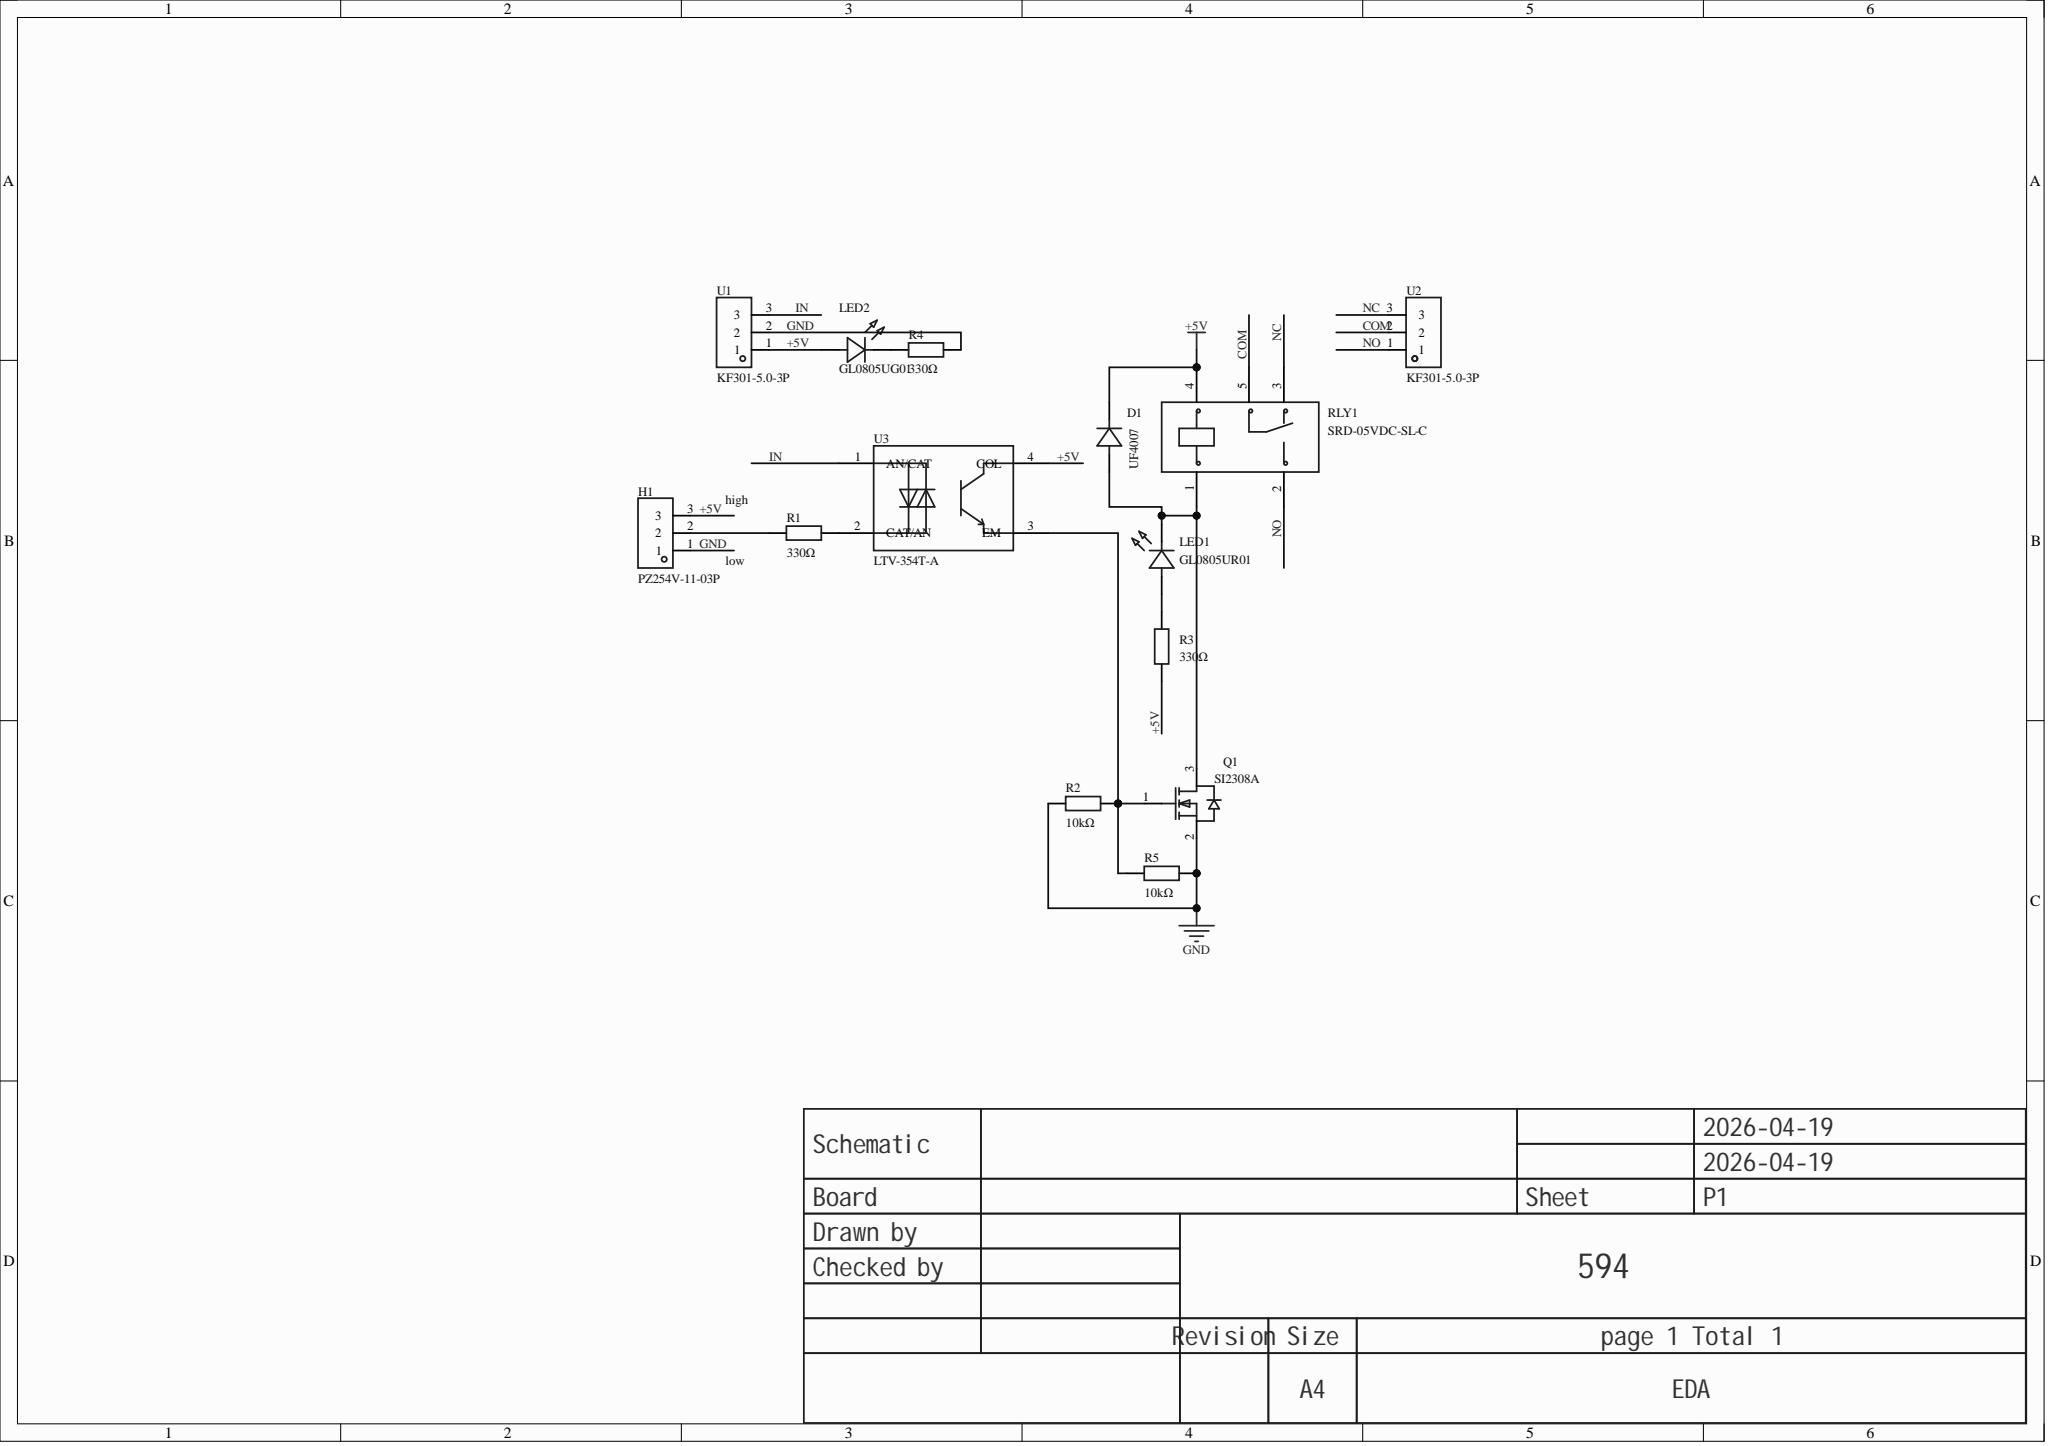Circuit board | Altium Designer | 14 parts | 12 nets
Bill of materials:
Comment,Description,Designator,Footprint,LibRef,Quantity
"UF4007","Diode configuration: -; forward voltage (Vf): 1.7V@1A; reverse breakdown voltage (Vr): 1kV; rectified current: 1A; reverse recovery time (Trr): 75ns;","D1","DO-41_BD2.4-L4.7-P8.70-D0.9-RD","UF4007_C960666","1"
"PZ254V-11-03P","","H1","HDR-TH_3P-P2.54-V-M_PZ254V-11-03P","PZ254V-11-03P","1"
"GL0805UR01","","LED1","LED0805-R-RD_RED","GL0805UR01","1"
"GL0805UG01","","LED2","LED0805-FD_GL0805UG01","GL0805UG01","1"
"SI2308A","Quantity: 1 N-channel; drain-source voltage (Vdss): 60V; continuous drain current (Id): 3A; on-resistance (RDS(on)): 80mΩ@10V; 95mΩ@4.5V; power dissipation (Pd): 1.25W; threshold voltage (Vgs(th)): 3V@250uA;","Q1","SOT-23-3_L2.9-W1.3-P1.90-LS2.4-BR","SI2308A","1"
"330Ω","Resistor type: thick film resistor; resistance: 330Ω; tolerance: ±1%; power: 100mW; max working voltage: 75V; temperature coefficient: ±100ppm/?;","R1, R3, R4","R0603","0603WAF3300T5E","3"
"10kΩ","Resistor type: thick film resistor; resistance: 10kΩ; tolerance: ±5%; power: 100mW; max working voltage: 75V; temperature coefficient: ±100ppm/?;","R2, R5","R0603","0603WAJ0103T5E","2"
"SRD-05VDC-SL-C","Coil voltage: 5V; contact form: changeover 1C (SPDT); contact rating (resistive load): -; max switching voltage: 250V@AC; max switching current: 15A;","RLY1","RELAY-TH_SRD-XXVDC-XL-C","SRD-05VDC-SL-C","1"
"KF301-5.0-3P","","U1, U2","CONN-TH_3P-P5.00_KF301-5.0-3P","KF301-5.0-3P","2"
"LTV-354T-A","Input type: AC,DC; forward voltage (Vf): 1.2V; output current: 50mA; isolation voltage (Vrms): 3.75kV; reverse breakdown voltage (Vr): -; load voltage: 35V; output channels: 1; collector-emitter saturation voltage (VCE(sat)): 100mV@20mA,1mA;","U3","SOP-4_L3.9-W4.4-P2.54-LS7.0-TL","LTV-354T-A","1"
Netlist (Protel format):
[
D1
DO-41_BD2.4-L4.7-P8.70-D0.9-RD
UF4007



]
[
H1
HDR-TH_3P-P2.54-V-M_PZ254V-11-03P
PZ254V-11-03P



]
[
LED1
LED0805-R-RD_RED
GL0805UR01



]
[
LED2
LED0805-FD_GL0805UG01
GL0805UG01



]
[
Q1
SOT-23-3_L2.9-W1.3-P1.90-LS2.4-BR
SI2308A



]
[
R1
R0603
330Ω



]
[
R2
R0603
10kΩ



]
[
R3
R0603
330Ω



]
[
R4
R0603
330Ω



]
[
R5
R0603
10kΩ



]
[
RLY1
RELAY-TH_SRD-XXVDC-XL-C
SRD-05VDC-SL-C



]
[
U1
CONN-TH_3P-P5.00_KF301-5.0-3P
KF301-5.0-3P



]
[
U2
CONN-TH_3P-P5.00_KF301-5.0-3P
KF301-5.0-3P



]
[
U3
SOP-4_L3.9-W4.4-P2.54-LS7.0-TL
LTV-354T-A



]
(
NO
RLY1-2
U2-1
)
(
NetR1_2
R1-2
U3-2
)
(
NetQ1_1
Q1-1
R2-2
R5-1
U3-3
)
(
NetLED2_2
LED2-2
R4-1
)
(
NetLED1_1
LED1-1
R3-2
)
(
NetH1_2
H1-2
R1-1
)
(
NetD1_2
D1-2
LED1-2
Q1-3
RLY1-1
)
(
NC
RLY1-3
U2-3
)
(
IN
U1-3
U3-1
)
(
GND
H1-1
Q1-2
R2-1
R4-2
R5-2
U1-2
)
(
COM
RLY1-5
U2-2
)
(
+5V
D1-1
H1-3
LED2-1
R3-1
RLY1-4
U1-1
U3-4
)